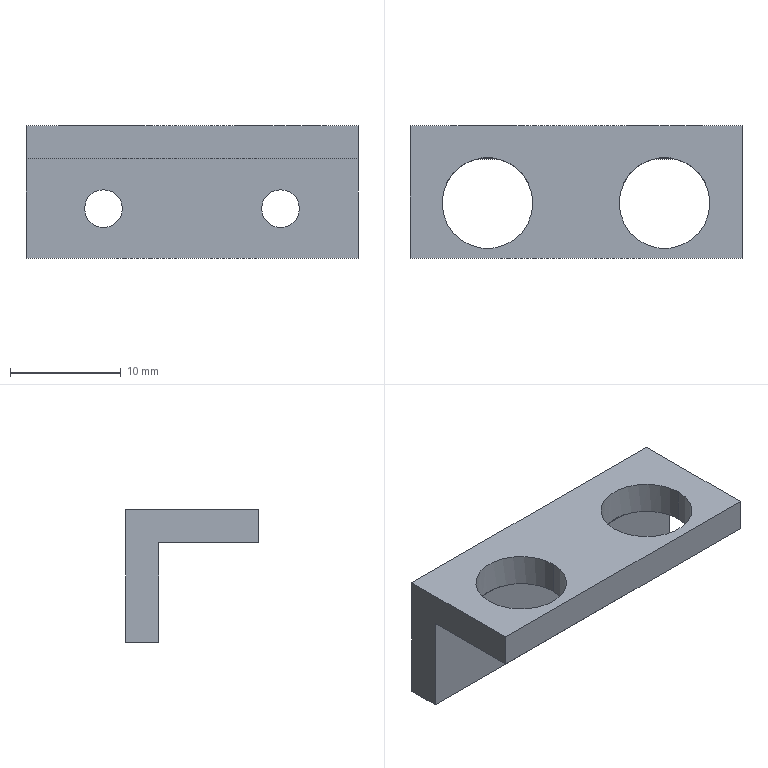NC program | NX | posted with a generic post | part box 30 x 12 x 12 mm
Lines 1 to 27 of 1871:
N10 G17 G21 G94 G90
(DRILLING , TOOL : ZXZ)
N12 T21 M6
N14 G54
N16 G17 G0 G90 X8. Y1.5 B0. C0. S3500 M3
N18 G43 Z30. H21
N20 G94 G81 G98 Z-1. F250. R3.
N22 X-8.
N24 G80
N26 G0 X-8. Y1.5 Z30.
N28 M5
(DRILLING_COPY_1 , TOOL : 3.4ZT)
N30 T13 M6
N32 G54
N34 G17 G0 G90 X-8. Y1.5 B0. C0. S2000 M3
N36 G43 Z30. H13
N38 G94 G83 G98 Z-5.521 F150. Q2. R3.
N40 X8.
N42 G80
N44 G0 X8. Y1.5 Z30.
N46 M5